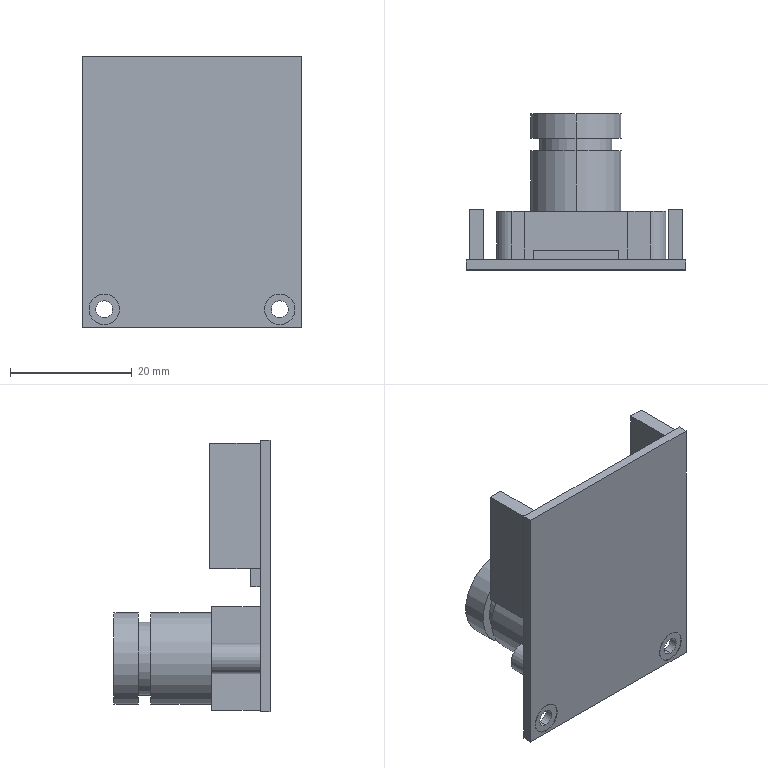Part | SolidWorks | features BaseBody 1 | 1 solid | 149 faces | box 36 x 25.6 x 44.5 mm | volume 8664 mm3 | plane 123 | cylinder 26 | commonest cylinder face diameters 5 x10 2 x4 2.8 x4 15 x4 9 x2 12 x2